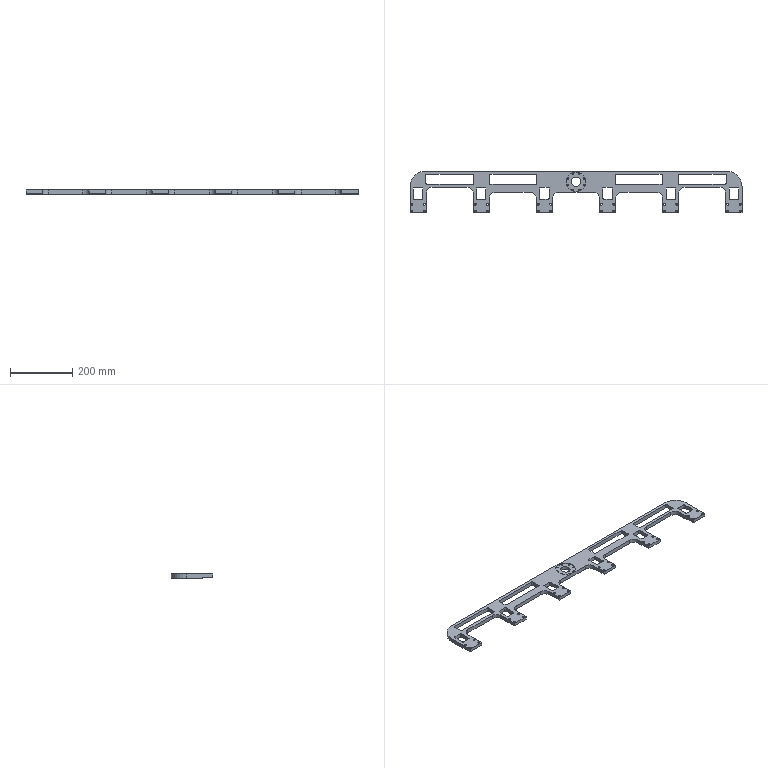CAM job | NX | 3-axis milling, drilling | part box 1068 x 134 x 13 mm | stock box 1076 x 142 x 15 mm
Tools:
number,name,description,diameter,corner_radius,flute_length,length,flutes
1,D63,Milling Tool-5 Parameters,63.0,0.0,50.0,75.0,2
7,D6A45,Milling Tool-5 Parameters,6.0,0.0,50.0,75.0,2
14,4.5ZT,Drilling Tool,4.5,0.0,35.0,50.0,2
15,6.5ZT,Drilling Tool,6.5,0.0,35.0,50.0,2
10,D10,Milling Tool-5 Parameters,10.0,0.0,50.0,75.0,2
6,D6,Milling Tool-5 Parameters,6.0,0.0,50.0,75.0,2
Operations:
program,operation,operation_type,tool,method,geometry_group,spindle_rpm,surface_speed,feed_per_tooth,feed_cut,feed_plunge,cut_length_mm,path_length_mm,cut_time_min,machine_time_min
1,FLOOR_WALL_COPY,VolumeBased25DMillingOperation,D63,METHOD,A,6500.0,1286.0,0.1154,1500.0,100.0,8681.192,8933.189,5.787,5.813
1,DRILLING_COPY_1,Operation,D6A45,METHOD,A,5000.0,94.0,0.025,250.0,0.0,100.0,1348.766,0.4,0.5249
1,DRILLING_COPY_COPY_1,Operation,4.5ZT,METHOD,A,2000.0,28.0,0.0625,250.0,0.0,146.815,526.106,0.5873,0.6252
1,DRILLING_COPY_COPY_COPY,Operation,6.5ZT,METHOD,A,2000.0,28.0,0.0625,250.0,0.0,303.245,1539.25,1.213,1.337
1,ZLEVEL_PROFILE_COPY_3,ZLevelMilling,D10,METHOD,A,9500.0,298.0,0.1842,3500.0,1000.0,24012.109,24835.709,6.947,7.029
1,ZLEVEL_PROFILE_COPY_2_COPY,ZLevelMilling,D10,METHOD,A,9500.0,298.0,0.1842,3500.0,1000.0,15268.987,16923.776,4.601,4.766
1,ZLEVEL_PROFILE_COPY_COPY_1,ZLevelMilling,D10,METHOD,A,9500.0,298.0,0.0789,1500.0,1000.0,3493.3,5397.398,2.456,2.646
1,FLOOR_WALL_1_COPY_1,VolumeBased25DMillingOperation,D10,METHOD,A,9500.0,298.0,0.1579,3000.0,1000.0,6128.989,7132.641,2.073,2.173
1,FLOOR_WALL_1_COPY_COPY,VolumeBased25DMillingOperation,D10,METHOD,A,9500.0,298.0,0.0789,1500.0,1000.0,1672.343,2569.495,1.122,1.211
1,HOLE_MILLING_COPY,CylinderMilling,D6,METHOD,A,9500.0,179.0,0.0737,1400.0,100.0,589.727,1252.539,0.4212,0.4875
1,ZLEVEL_PROFILE_COPY_1_COPY,ZLevelMilling,D6,METHOD,A,9500.0,179.0,0.0868,1650.0,1000.0,3669.553,8390.359,2.486,2.958
1,PLANAR_MILL_COPY_1,PlanarMilling,D6A45,METHOD,A,9500.0,179.0,0.0737,1400.0,100.0,3185.084,5215.129,2.275,2.478
1,PLANAR_MILL_COPY_COPY,PlanarMilling,D6A45,METHOD,A,9500.0,179.0,0.0737,1400.0,100.0,798.754,4008.097,0.5705,0.8915
1,ZLEVEL_PROFILE_COPY_3_COPY,ZLevelMilling,D10,METHOD,A,9500.0,298.0,0.0632,1200.0,1000.0,7387.068,8140.732,6.162,6.237
2,FLOOR_WALL_COPY_COPY,VolumeBased25DMillingOperation,D63,METHOD,A,6500.0,1286.0,0.1154,1500.0,100.0,5738.792,5990.789,3.826,3.851
2,DRILLING_COPY_1_COPY,Operation,D6A45,METHOD,A,5000.0,94.0,0.025,250.0,0.0,32.0,477.267,0.128,0.1725
2,DRILLING_COPY_COPY_COPY_COPY,Operation,6.5ZT,METHOD,A,2000.0,28.0,0.0625,250.0,0.0,151.622,716.511,0.6065,0.663
2,ZLEVEL_PROFILE_COPY_3_COPY_1,ZLevelMilling,D10,METHOD,A,9500.0,298.0,0.1842,3500.0,1000.0,16147.927,16971.527,4.702,4.784
2,ZLEVEL_PROFILE_COPY_2_COPY_COPY,ZLevelMilling,D10,METHOD,A,9500.0,298.0,0.1842,3500.0,1000.0,11573.219,12511.37,3.443,3.537
2,ZLEVEL_PROFILE_COPY_COPY_1_COPY,ZLevelMilling,D10,METHOD,A,9500.0,298.0,0.0789,1500.0,1000.0,2543.289,3165.489,1.753,1.815
2,FLOOR_WALL_1_COPY_1_COPY,VolumeBased25DMillingOperation,D10,METHOD,A,9500.0,298.0,0.1579,3000.0,1000.0,3064.495,3463.194,1.036,1.076
2,FLOOR_WALL_1_COPY_COPY_COPY,VolumeBased25DMillingOperation,D10,METHOD,A,9500.0,298.0,0.0789,1500.0,1000.0,836.172,1194.976,0.5608,0.5967
2,ZLEVEL_PROFILE_COPY_1_COPY_COPY,ZLevelMilling,D6,METHOD,A,9500.0,179.0,0.0868,1650.0,1000.0,2446.706,5334.796,1.657,1.946
2,PLANAR_MILL_COPY_1_COPY,PlanarMilling,D6A45,METHOD,A,9500.0,179.0,0.0737,1400.0,100.0,2047.85,3048.787,1.463,1.563
2,PLANAR_MILL_COPY_COPY_COPY,PlanarMilling,D6A45,METHOD,A,9500.0,179.0,0.0737,1400.0,100.0,399.377,1481.107,0.2853,0.3934
2,ZLEVEL_PROFILE_COPY_3_COPY_COPY,ZLevelMilling,D10,METHOD,A,9500.0,298.0,0.0632,1200.0,1000.0,4967.336,5722.036,4.146,4.221